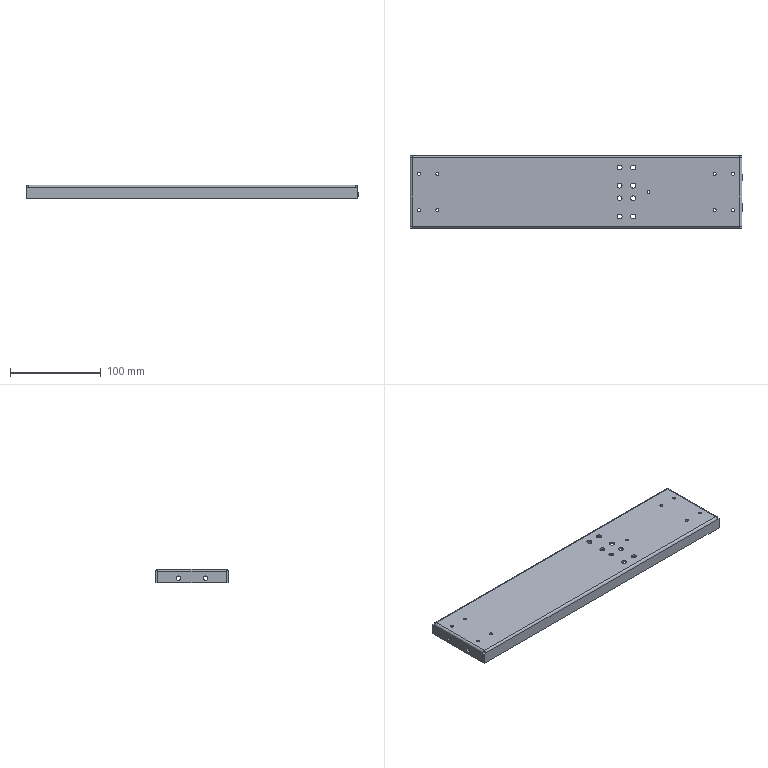Part | SolidWorks | features HoleWzd 4, EdgeFlange 2, MirrorPattern 2, FlatPattern 1, ICE 1, SMBaseFlange 1, SheetMetal 1 | 1 solid | 84 faces | box 366 x 80 x 15 mm | volume 79720 mm3 | cylinder 50 | plane 34 | commonest cylinder face diameters 3.2 x16 5.5 x16 5 x8 0.8 x4 4.8 x4 3 x2